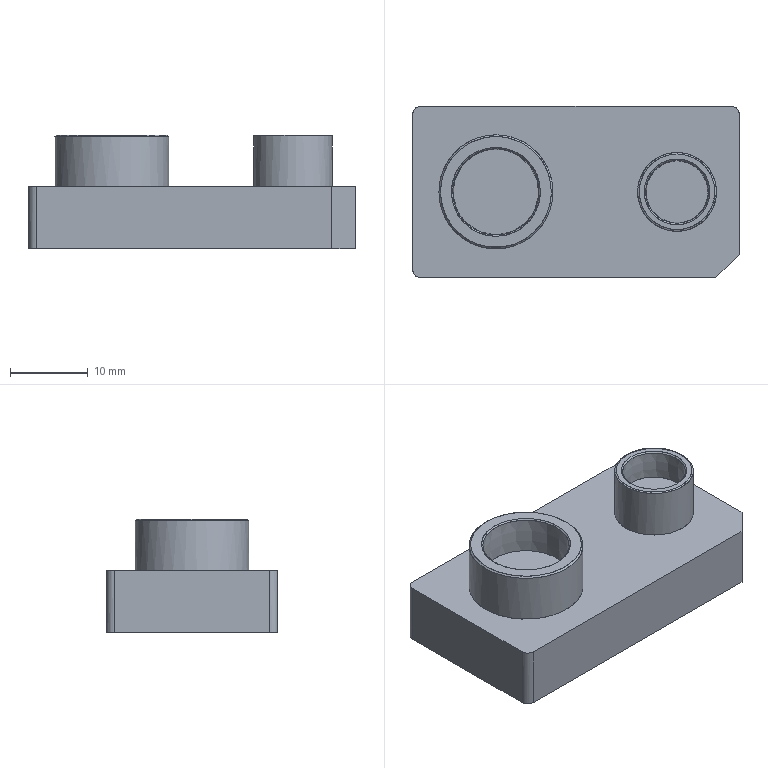NC program | PowerMill | posted by the shop | part box 42 x 22 x 14.621 mm
Lines 1 to 1559 of 126517:
%
G40 G49 G17 G80
( TOOL ID   D10C_1_1 )
( TOOL DIA. 10. TIP RAD 0 LENGTH 70.08 )
( Z = -.069 )
T1 M6
T2
G91 G28 Z0
G0 G90 G54
M08
S8000 M3
G0 X0 Y0 M8
G43 Z10.2 H1
X28.78 Y13.78
Z1.131
G1 Z-.069 F6000
X23.78 F10000
X-23.78
Y8.268
X23.78
Y2.756
X-23.78
Y-2.756
X23.78
Y-8.268
X-23.78
Y-13.78
X23.78
X28.78
G0 Z10.2
X.22 Y0
Z9.881
X31.126 Y5.112
Z.698
G1 Z-.502 F6000
X30.598 F10000
G3 X25.851 Y.364 I0 J-4.748
G1 Y-14.113
G2 X24.851 Y-15.113 I-1. J0
G1 X-24.411
G2 X-25.411 Y-14.113 I0 J1.
G1 Y14.113
G2 X-24.411 Y15.113 I1. J0
G1 X24.851
G2 X25.851 Y14.113 I0 J-1.
G1 Y.364
X23.346 Y.387
X23.339 Y-.387
X23.288 Y-1.16
X23.165 Y-1.934
X22.993 Y-2.707
X22.744 Y-3.48
X22.439 Y-4.254
X22.039 Y-5.027
X21.574 Y-5.801
X20.989 Y-6.574
X20.329 Y-7.311
X19.556 Y-8.014
X18.782 Y-8.573
X18.009 Y-9.061
X17.235 Y-9.439
X16.701 Y-9.668
X15.689 Y-9.993
X14.915 Y-10.175
X14.142 Y-10.285
X13.368 Y-10.347
X12.595 Y-10.339
X11.821 Y-10.286
X11.048 Y-10.16
X10.275 Y-9.988
X9.501 Y-9.737
X8.728 Y-9.431
X7.954 Y-9.037
X7.181 Y-8.561
X6.581 Y-8.121
X5.722 Y-7.348
X5.001 Y-6.574
X4.426 Y-5.801
X4.087 Y-5.268
X3.561 Y-4.254
X3.314 Y-3.65
X3.007 Y-2.707
X2.837 Y-1.934
X2.712 Y-1.16
X2.661 Y-.387
X2.654 Y.387
X2.295
Y-.387
X2.248 Y-1.16
X2.153 Y-1.934
X2.008 Y-2.707
X1.812 Y-3.48
X1.562 Y-4.254
X1.256 Y-5.027
X.993 Y-5.601
X.458 Y-6.574
X-.052 Y-7.348
X-.553 Y-8.001
X-1.327 Y-8.853
X-2.1 Y-9.578
X-2.874 Y-10.193
X-3.647 Y-10.713
X-4.421 Y-11.154
X-5.194 Y-11.527
X-6.381 Y-11.988
X-7.514 Y-12.294
X-8.288 Y-12.445
X-9.061 Y-12.546
X-9.835 Y-12.599
X-10.608 Y-12.605
X-11.381 Y-12.563
X-12.155 Y-12.473
X-12.928 Y-12.334
X-14.227 Y-11.988
X-15.249 Y-11.598
X-16.063 Y-11.215
X-16.795 Y-10.809
X-17.569 Y-10.31
X-18.342 Y-9.721
X-19.116 Y-9.021
X-19.889 Y-8.196
X-20.557 Y-7.348
X-21.066 Y-6.574
X-21.436 Y-5.929
X-21.865 Y-5.027
X-22.209 Y-4.156
X-22.421 Y-3.48
X-22.617 Y-2.707
X-22.762 Y-1.934
X-22.857 Y-1.16
X-22.904 Y-.387
Y.387
X-22.857 Y1.16
X-22.762 Y1.934
X-22.617 Y2.707
X-22.421 Y3.48
X-22.209 Y4.156
X-21.865 Y5.027
X-21.436 Y5.929
X-21.066 Y6.574
X-20.663 Y7.191
X-19.955 Y8.121
X-19.238 Y8.894
X-18.406 Y9.668
X-17.569 Y10.31
X-16.795 Y10.809
X-16.063 Y11.215
X-15.249 Y11.598
X-14.227 Y11.988
X-12.928 Y12.334
X-12.155 Y12.473
X-11.381 Y12.563
X-10.608 Y12.605
X-9.835 Y12.599
X-9.061 Y12.546
X-8.288 Y12.445
X-7.514 Y12.294
X-6.381 Y11.988
X-5.194 Y11.527
X-4.421 Y11.154
X-3.647 Y10.713
X-2.874 Y10.193
X-2.203 Y9.668
X-1.327 Y8.853
X-.653 Y8.121
X-.052 Y7.348
X.458 Y6.574
X.89 Y5.801
X1.256 Y5.027
X1.562 Y4.254
X1.767 Y3.646
X2.008 Y2.707
X2.153 Y1.934
X2.248 Y1.16
X2.295 Y.387
X2.654
X2.718 Y1.16
X2.829 Y1.934
X3.013 Y2.707
X3.249 Y3.48
X3.57 Y4.254
X4.087 Y5.268
X4.861 Y6.397
X5.634 Y7.271
X6.407 Y7.974
X7.181 Y8.562
X7.715 Y8.894
X8.728 Y9.431
X9.501 Y9.737
X10.275 Y9.988
X11.048 Y10.161
X11.821 Y10.286
X12.595 Y10.338
X13.368 Y10.347
X14.142 Y10.281
X14.915 Y10.175
X15.689 Y9.989
X16.462 Y9.758
X17.235 Y9.44
X18.009 Y9.061
X18.782 Y8.586
X19.42 Y8.121
X20.293 Y7.348
X20.99 Y6.574
X21.574 Y5.801
X22.051 Y5.027
X22.432 Y4.254
X22.751 Y3.48
X22.985 Y2.707
X23.171 Y1.934
X23.28 Y1.16
X23.346 Y.387
X25.851 Y.364
G0 Z3.315
G1 X31.126 Y5.112
G0 Z.315
G1 Z-.885 F6000
X30.598 F10000
G3 X25.851 Y.364 I0 J-4.748
G1 Y-14.113
G2 X24.851 Y-15.113 I-1. J0
G1 X-24.411
G2 X-25.411 Y-14.113 I0 J1.
G1 Y14.113
G2 X-24.411 Y15.113 I1. J0
G1 X24.851
G2 X25.851 Y14.113 I0 J-1.
G1 Y.364
X23.346 Y.387
X23.339 Y-.387
X23.288 Y-1.16
X23.165 Y-1.934
X22.993 Y-2.707
X22.744 Y-3.48
X22.439 Y-4.254
X22.039 Y-5.027
X21.574 Y-5.801
X20.989 Y-6.574
X20.329 Y-7.311
X19.556 Y-8.014
X18.782 Y-8.573
X18.009 Y-9.061
X17.235 Y-9.44
X16.701 Y-9.668
X15.689 Y-9.993
X14.915 Y-10.175
X14.142 Y-10.285
X13.368 Y-10.347
X12.595 Y-10.339
X11.821 Y-10.286
X11.048 Y-10.16
X10.275 Y-9.988
X9.501 Y-9.737
X8.728 Y-9.431
X7.954 Y-9.037
X7.181 Y-8.561
X6.581 Y-8.121
X5.722 Y-7.348
X5.001 Y-6.574
X4.426 Y-5.801
X4.087 Y-5.268
X3.561 Y-4.254
X3.314 Y-3.65
X3.007 Y-2.707
X2.837 Y-1.934
X2.712 Y-1.16
X2.661 Y-.387
X2.654 Y.387
X2.295
Y-.387
X2.248 Y-1.16
X2.153 Y-1.934
X2.008 Y-2.707
X1.812 Y-3.48
X1.562 Y-4.254
X1.256 Y-5.027
X.993 Y-5.601
X.458 Y-6.574
X-.052 Y-7.348
X-.553 Y-8.001
X-1.327 Y-8.853
X-2.1 Y-9.578
X-2.874 Y-10.193
X-3.647 Y-10.713
X-4.421 Y-11.154
X-5.194 Y-11.527
X-6.381 Y-11.988
X-7.514 Y-12.294
X-8.288 Y-12.445
X-9.061 Y-12.546
X-9.835 Y-12.599
X-10.608 Y-12.605
X-11.381 Y-12.563
X-12.155 Y-12.473
X-12.928 Y-12.334
X-14.227 Y-11.988
X-15.249 Y-11.598
X-16.063 Y-11.215
X-16.795 Y-10.809
X-17.569 Y-10.31
X-18.342 Y-9.721
X-19.116 Y-9.021
X-19.889 Y-8.196
X-20.557 Y-7.348
X-21.066 Y-6.574
X-21.436 Y-5.929
X-21.865 Y-5.027
X-22.209 Y-4.156
X-22.421 Y-3.48
X-22.617 Y-2.707
X-22.762 Y-1.934
X-22.857 Y-1.16
X-22.904 Y-.387
Y.387
X-22.857 Y1.16
X-22.762 Y1.934
X-22.617 Y2.707
X-22.421 Y3.48
X-22.209 Y4.156
X-21.865 Y5.027
X-21.436 Y5.929
X-21.066 Y6.574
X-20.663 Y7.191
X-19.955 Y8.121
X-19.238 Y8.894
X-18.406 Y9.668
X-17.569 Y10.31
X-16.795 Y10.809
X-16.063 Y11.215
X-15.249 Y11.598
X-14.227 Y11.988
X-12.928 Y12.334
X-12.155 Y12.473
X-11.381 Y12.563
X-10.608 Y12.605
X-9.835 Y12.599
X-9.061 Y12.546
X-8.288 Y12.445
X-7.514 Y12.294
X-6.381 Y11.988
X-5.194 Y11.527
X-4.421 Y11.154
X-3.647 Y10.713
X-2.874 Y10.193
X-2.203 Y9.668
X-1.327 Y8.853
X-.653 Y8.121
X-.052 Y7.348
X.458 Y6.574
X.89 Y5.801
X1.256 Y5.027
X1.562 Y4.254
X1.767 Y3.646
X2.008 Y2.707
X2.153 Y1.934
X2.248 Y1.16
X2.295 Y.387
X2.654
X2.718 Y1.16
X2.829 Y1.934
X3.013 Y2.707
X3.249 Y3.48
X3.57 Y4.254
X4.087 Y5.269
X4.861 Y6.397
X5.634 Y7.271
X6.407 Y7.974
X7.181 Y8.562
X7.715 Y8.894
X8.728 Y9.431
X9.501 Y9.737
X10.275 Y9.988
X11.048 Y10.161
X11.821 Y10.286
X12.595 Y10.338
X13.368 Y10.347
X14.142 Y10.281
X14.915 Y10.175
X15.689 Y9.989
X16.462 Y9.758
X17.235 Y9.44
X18.009 Y9.061
X18.782 Y8.586
X19.42 Y8.121
X20.293 Y7.348
X20.99 Y6.574
X21.574 Y5.801
X22.051 Y5.027
X22.432 Y4.254
X22.751 Y3.48
X22.985 Y2.707
X23.171 Y1.934
X23.28 Y1.16
X23.346 Y.387
X25.851 Y.364
G0 Z2.932
G1 X31.126 Y5.112
G0 Z-.068
G1 Z-1.268 F6000
X30.598 F10000
G3 X25.851 Y.364 I0 J-4.748
G1 Y-14.113
G2 X24.851 Y-15.113 I-1. J0
G1 X-24.411
G2 X-25.411 Y-14.113 I0 J1.
G1 Y14.113
G2 X-24.411 Y15.113 I1. J0
G1 X24.851
G2 X25.851 Y14.113 I0 J-1.
G1 Y.364
X23.346 Y.387
X23.339 Y-.387
X23.288 Y-1.16
X23.165 Y-1.934
X22.993 Y-2.707
X22.744 Y-3.48
X22.439 Y-4.254
X22.039 Y-5.027
X21.574 Y-5.801
X20.989 Y-6.574
X20.329 Y-7.311
X19.556 Y-8.014
X18.782 Y-8.573
X18.009 Y-9.061
X17.235 Y-9.44
X16.701 Y-9.668
X15.689 Y-9.993
X14.915 Y-10.175
X14.142 Y-10.285
X13.368 Y-10.347
X12.595 Y-10.339
X11.821 Y-10.286
X11.048 Y-10.16
X10.275 Y-9.988
X9.501 Y-9.737
X8.728 Y-9.431
X7.954 Y-9.037
X7.181 Y-8.561
X6.581 Y-8.121
X5.722 Y-7.348
X5.001 Y-6.574
X4.426 Y-5.801
X4.087 Y-5.268
X3.561 Y-4.254
X3.314 Y-3.65
X3.007 Y-2.707
X2.837 Y-1.934
X2.712 Y-1.16
X2.661 Y-.387
X2.654 Y.387
X2.295
Y-.387
X2.248 Y-1.16
X2.153 Y-1.934
X2.008 Y-2.707
X1.812 Y-3.48
X1.562 Y-4.254
X1.256 Y-5.027
X.993 Y-5.601
X.458 Y-6.574
X-.052 Y-7.348
X-.553 Y-8.001
X-1.327 Y-8.853
X-2.1 Y-9.578
X-2.874 Y-10.193
X-3.647 Y-10.713
X-4.421 Y-11.154
X-5.194 Y-11.527
X-6.381 Y-11.988
X-7.514 Y-12.294
X-8.288 Y-12.445
X-9.061 Y-12.546
X-9.835 Y-12.599
X-10.608 Y-12.605
X-11.381 Y-12.563
X-12.155 Y-12.473
X-12.928 Y-12.334
X-14.227 Y-11.988
X-15.249 Y-11.598
X-16.063 Y-11.215
X-16.795 Y-10.809
X-17.569 Y-10.31
X-18.342 Y-9.721
X-19.116 Y-9.021
X-19.889 Y-8.196
X-20.557 Y-7.348
X-21.066 Y-6.574
X-21.436 Y-5.929
X-21.865 Y-5.027
X-22.209 Y-4.156
X-22.421 Y-3.48
X-22.617 Y-2.707
X-22.762 Y-1.934
X-22.857 Y-1.16
X-22.904 Y-.387
Y.387
X-22.857 Y1.16
X-22.762 Y1.934
X-22.617 Y2.707
X-22.421 Y3.48
X-22.209 Y4.156
X-21.865 Y5.027
X-21.436 Y5.929
X-21.066 Y6.574
X-20.663 Y7.191
X-19.955 Y8.121
X-19.238 Y8.894
X-18.406 Y9.668
X-17.569 Y10.31
X-16.795 Y10.809
X-16.063 Y11.215
X-15.249 Y11.598
X-14.227 Y11.988
X-12.928 Y12.334
X-12.155 Y12.473
X-11.381 Y12.563
X-10.608 Y12.605
X-9.835 Y12.599
X-9.061 Y12.546
X-8.288 Y12.445
X-7.514 Y12.294
X-6.381 Y11.988
X-5.194 Y11.527
X-4.421 Y11.154
X-3.647 Y10.713
X-2.874 Y10.193
X-2.203 Y9.668
X-1.327 Y8.853
X-.653 Y8.121
X-.052 Y7.348
X.458 Y6.574
X.89 Y5.801
X1.256 Y5.027
X1.562 Y4.254
X1.767 Y3.646
X2.008 Y2.707
X2.153 Y1.934
X2.248 Y1.16
X2.295 Y.387
X2.654
X2.718 Y1.16
X2.829 Y1.934
X3.013 Y2.707
X3.249 Y3.48
X3.57 Y4.254
X4.087 Y5.269
X4.861 Y6.397
X5.634 Y7.271
X6.407 Y7.974
X7.181 Y8.562
X7.715 Y8.894
X8.728 Y9.431
X9.501 Y9.737
X10.275 Y9.988
X11.048 Y10.161
X11.821 Y10.286
X12.595 Y10.338
X13.368 Y10.347
X14.142 Y10.281
X14.915 Y10.175
X15.689 Y9.989
X16.462 Y9.758
X17.235 Y9.44
X18.009 Y9.061
X18.782 Y8.586
X19.42 Y8.121
X20.293 Y7.348
X20.99 Y6.574
X21.574 Y5.801
X22.051 Y5.027
X22.432 Y4.254
X22.751 Y3.48
X22.985 Y2.707
X23.171 Y1.934
X23.28 Y1.16
X23.346 Y.387
X25.851 Y.364
G0 Z2.549
G1 X31.126 Y5.112
G0 Z-.451
G1 Z-1.651 F6000
X30.598 F10000
G3 X25.851 Y.364 I0 J-4.748
G1 Y-14.113
G2 X24.851 Y-15.113 I-1. J0
G1 X-24.411
G2 X-25.411 Y-14.113 I0 J1.
G1 Y14.113
G2 X-24.411 Y15.113 I1. J0
G1 X24.851
G2 X25.851 Y14.113 I0 J-1.
G1 Y.364
X23.346 Y.387
X23.339 Y-.387
X23.288 Y-1.16
X23.165 Y-1.934
X22.993 Y-2.707
X22.744 Y-3.48
X22.439 Y-4.254
X22.039 Y-5.027
X21.574 Y-5.801
X20.989 Y-6.574
X20.329 Y-7.311
X19.556 Y-8.014
X18.782 Y-8.573
X18.009 Y-9.061
X17.235 Y-9.44
X16.701 Y-9.668
X15.689 Y-9.993
X14.915 Y-10.175
X14.142 Y-10.285
X13.368 Y-10.347
X12.595 Y-10.339
X11.821 Y-10.286
X11.048 Y-10.16
X10.275 Y-9.988
X9.501 Y-9.737
X8.728 Y-9.431
X7.954 Y-9.037
X7.181 Y-8.561
X6.581 Y-8.121
X5.722 Y-7.348
X5.001 Y-6.574
X4.426 Y-5.801
X4.087 Y-5.269
X3.561 Y-4.254
X3.314 Y-3.65
X3.007 Y-2.707
X2.837 Y-1.934
X2.712 Y-1.16
X2.661 Y-.387
X2.654 Y.387
X2.295
Y-.387
X2.248 Y-1.16
X2.153 Y-1.934
X2.008 Y-2.707
X1.812 Y-3.48
X1.562 Y-4.254
X1.256 Y-5.027
X.993 Y-5.601
X.458 Y-6.574
X-.052 Y-7.348
X-.553 Y-8.001
X-1.327 Y-8.853
X-2.1 Y-9.578
X-2.874 Y-10.193
X-3.647 Y-10.713
X-4.421 Y-11.154
X-5.194 Y-11.527
X-6.381 Y-11.988
X-7.514 Y-12.294
X-8.288 Y-12.445
X-9.061 Y-12.546
X-9.835 Y-12.599
X-10.608 Y-12.605
X-11.381 Y-12.563
X-12.155 Y-12.473
X-12.928 Y-12.334
X-14.227 Y-11.988
X-15.249 Y-11.598
X-16.063 Y-11.215
X-16.795 Y-10.809
X-17.569 Y-10.31
X-18.342 Y-9.721
X-19.116 Y-9.021
X-19.889 Y-8.196
X-20.557 Y-7.348
X-21.066 Y-6.574
X-21.436 Y-5.929
X-21.865 Y-5.027
X-22.209 Y-4.156
X-22.421 Y-3.48
X-22.617 Y-2.707
X-22.762 Y-1.934
X-22.857 Y-1.16
X-22.904 Y-.387
Y.387
X-22.857 Y1.16
X-22.762 Y1.934
X-22.617 Y2.707
X-22.421 Y3.48
X-22.209 Y4.156
X-21.865 Y5.027
X-21.436 Y5.929
X-21.066 Y6.574
X-20.663 Y7.191
X-19.955 Y8.121
X-19.238 Y8.894
X-18.406 Y9.668
X-17.569 Y10.31
X-16.795 Y10.809
X-16.063 Y11.215
X-15.249 Y11.598
X-14.227 Y11.988
X-12.928 Y12.334
X-12.155 Y12.473
X-11.381 Y12.563
X-10.608 Y12.605
X-9.835 Y12.599
X-9.061 Y12.546
X-8.288 Y12.445
X-7.514 Y12.294
X-6.381 Y11.988
X-5.194 Y11.527
X-4.421 Y11.154
X-3.647 Y10.713
X-2.874 Y10.193
X-2.203 Y9.668
X-1.327 Y8.853
X-.653 Y8.121
X-.052 Y7.348
X.458 Y6.574
X.89 Y5.801
X1.256 Y5.027
X1.562 Y4.254
X1.767 Y3.646
X2.008 Y2.707
X2.153 Y1.934
X2.248 Y1.16
X2.295 Y.387
X2.654
X2.718 Y1.16
X2.829 Y1.934
X3.013 Y2.707
X3.249 Y3.48
X3.57 Y4.254
X4.087 Y5.269
X4.861 Y6.397
X5.634 Y7.271
X6.407 Y7.974
X7.181 Y8.562
X7.715 Y8.894
X8.728 Y9.431
X9.501 Y9.737
X10.275 Y9.988
X11.048 Y10.161
X11.821 Y10.286
X12.595 Y10.338
X13.368 Y10.347
X14.142 Y10.281
X14.915 Y10.175
X15.689 Y9.989
X16.462 Y9.758
X17.235 Y9.44
X18.009 Y9.061
X18.782 Y8.586
X19.42 Y8.121
X20.293 Y7.348
X20.99 Y6.574
X21.574 Y5.801
X22.051 Y5.027
X22.432 Y4.254
X22.751 Y3.48
X22.985 Y2.707
X23.171 Y1.934
X23.28 Y1.16
X23.346 Y.387
X25.851 Y.364
G0 Z2.166
G1 X31.126 Y5.112
G0 Z-.834
G1 Z-2.034 F6000
X30.598 F10000
G3 X25.851 Y.364 I0 J-4.748
G1 Y-14.113
G2 X24.851 Y-15.113 I-1. J0
G1 X-24.411
G2 X-25.411 Y-14.113 I0 J1.
G1 Y14.113
G2 X-24.411 Y15.113 I1. J0
G1 X24.851
G2 X25.851 Y14.113 I0 J-1.
G1 Y.364
X23.346 Y.387
X23.339 Y-.387
X23.288 Y-1.16
X23.165 Y-1.934
X22.993 Y-2.707
X22.744 Y-3.48
X22.439 Y-4.254
X22.039 Y-5.027
X21.574 Y-5.801
X20.989 Y-6.574
X20.329 Y-7.311
X19.556 Y-8.014
X18.782 Y-8.573
X18.009 Y-9.061
X17.235 Y-9.44
X16.701 Y-9.668
X15.689 Y-9.993
X14.915 Y-10.175
X14.142 Y-10.285
X13.368 Y-10.347
X12.595 Y-10.339
X11.821 Y-10.286
X11.048 Y-10.16
X10.275 Y-9.988
X9.501 Y-9.737
X8.728 Y-9.431
X7.954 Y-9.037
X7.181 Y-8.561
X6.581 Y-8.121
X5.722 Y-7.348
X5.001 Y-6.574
X4.426 Y-5.801
X4.087 Y-5.269
X3.561 Y-4.254
X3.314 Y-3.65
X3.007 Y-2.707
X2.837 Y-1.934
X2.712 Y-1.16
X2.661 Y-.387
X2.654 Y.387
X2.295
Y-.387
X2.248 Y-1.16
X2.153 Y-1.934
X2.008 Y-2.707
X1.812 Y-3.48
X1.562 Y-4.254
X1.256 Y-5.027
X.993 Y-5.601
X.458 Y-6.574
X-.052 Y-7.348
X-.553 Y-8.001
X-1.327 Y-8.853
X-2.1 Y-9.578
X-2.874 Y-10.193
X-3.647 Y-10.713
X-4.421 Y-11.154
X-5.194 Y-11.527
X-6.381 Y-11.988
X-7.514 Y-12.294
X-8.288 Y-12.445
X-9.061 Y-12.546
X-9.835 Y-12.599
X-10.608 Y-12.605
X-11.381 Y-12.563
X-12.155 Y-12.473
X-12.928 Y-12.334
X-14.227 Y-11.988
X-15.249 Y-11.598
X-16.063 Y-11.215
X-16.795 Y-10.809
X-17.569 Y-10.31
X-18.342 Y-9.721
X-19.116 Y-9.021
X-19.889 Y-8.196
X-20.557 Y-7.348
X-21.066 Y-6.574
X-21.436 Y-5.929
X-21.865 Y-5.027
X-22.209 Y-4.156
X-22.421 Y-3.48
X-22.617 Y-2.707
X-22.762 Y-1.934
X-22.857 Y-1.16
X-22.904 Y-.387
Y.387
X-22.857 Y1.16
X-22.762 Y1.934
X-22.617 Y2.707
X-22.421 Y3.48
X-22.209 Y4.156
X-21.865 Y5.027
X-21.436 Y5.929
X-21.066 Y6.574
X-20.663 Y7.191
X-19.955 Y8.121
X-19.238 Y8.894
X-18.406 Y9.668
X-17.569 Y10.31
X-16.795 Y10.809
X-16.063 Y11.215
X-15.249 Y11.598
X-14.227 Y11.988
X-12.928 Y12.334
X-12.155 Y12.473
X-11.381 Y12.563
X-10.608 Y12.605
X-9.835 Y12.599
X-9.061 Y12.546
X-8.288 Y12.445
X-7.514 Y12.294
X-6.381 Y11.988
X-5.194 Y11.527
X-4.421 Y11.154
X-3.647 Y10.713
X-2.874 Y10.193
X-2.203 Y9.668
X-1.327 Y8.853
X-.653 Y8.121
X-.052 Y7.348
X.458 Y6.574
X.89 Y5.801
X1.256 Y5.027
X1.562 Y4.254
X1.767 Y3.646
X2.008 Y2.707
X2.153 Y1.934
X2.248 Y1.16
X2.295 Y.387
X2.654
X2.718 Y1.16
X2.829 Y1.934
X3.013 Y2.707
X3.249 Y3.48
X3.57 Y4.254
X4.087 Y5.269
X4.861 Y6.397
X5.634 Y7.271
X6.407 Y7.974
X7.181 Y8.562
X7.715 Y8.894
X8.728 Y9.431
X9.501 Y9.737
X10.275 Y9.988
X11.048 Y10.161
X11.821 Y10.286
X12.595 Y10.338
X13.368 Y10.347
X14.142 Y10.281
X14.915 Y10.175
X15.689 Y9.989
X16.462 Y9.758
X17.235 Y9.44
X18.009 Y9.061
X18.782 Y8.586
X19.42 Y8.121
X20.293 Y7.348
X20.99 Y6.574
X21.574 Y5.801
X22.051 Y5.027
X22.432 Y4.254
X22.751 Y3.48
X22.985 Y2.707
X23.171 Y1.934
X23.28 Y1.16
X23.346 Y.387
X25.851 Y.364
G0 Z1.783
G1 X31.126 Y5.112
G0 Z-1.217
G1 Z-2.417 F6000
X30.598 F10000
G3 X25.851 Y.364 I0 J-4.748
G1 Y-14.113
G2 X24.851 Y-15.113 I-1. J0
G1 X-24.411
G2 X-25.411 Y-14.113 I0 J1.
G1 Y14.113
G2 X-24.411 Y15.113 I1. J0
G1 X24.851
G2 X25.851 Y14.113 I0 J-1.
G1 Y.364
X23.346 Y.387
X23.339 Y-.387
X23.288 Y-1.16
X23.165 Y-1.934
X22.993 Y-2.707
X22.744 Y-3.48
X22.439 Y-4.254
X22.039 Y-5.027
X21.574 Y-5.801
X20.989 Y-6.574
X20.329 Y-7.311
X19.556 Y-8.014
X18.782 Y-8.573
X18.009 Y-9.061
X17.235 Y-9.44
X16.701 Y-9.668
X15.689 Y-9.993
X14.915 Y-10.175
X14.142 Y-10.285
X13.368 Y-10.347
X12.595 Y-10.339
X11.821 Y-10.286
X11.048 Y-10.16
X10.275 Y-9.988
X9.501 Y-9.737
X8.728 Y-9.431
X7.954 Y-9.037
X7.181 Y-8.561
X6.581 Y-8.121
X5.722 Y-7.348
X5.001 Y-6.574
X4.426 Y-5.801
X4.087 Y-5.269
X3.561 Y-4.254
X3.314 Y-3.65
X3.007 Y-2.707
X2.837 Y-1.934
X2.712 Y-1.16
X2.661 Y-.387
X2.654 Y.387
X2.295
Y-.387
X2.248 Y-1.16
X2.153 Y-1.934
X2.008 Y-2.707
X1.812 Y-3.48
X1.562 Y-4.254
X1.256 Y-5.027
X.993 Y-5.601
X.458 Y-6.574
X-.052 Y-7.348
X-.553 Y-8.001
X-1.327 Y-8.853
X-2.1 Y-9.578
X-2.874 Y-10.193
X-3.647 Y-10.713
X-4.421 Y-11.154
X-5.194 Y-11.527
X-6.381 Y-11.988
X-7.514 Y-12.294
X-8.288 Y-12.445
X-9.061 Y-12.546
X-9.835 Y-12.599
X-10.608 Y-12.605
X-11.381 Y-12.563
X-12.155 Y-12.473
X-12.928 Y-12.334
X-14.227 Y-11.988
X-15.249 Y-11.598
X-16.063 Y-11.215
X-16.795 Y-10.809
X-17.569 Y-10.31
X-18.342 Y-9.721
X-19.116 Y-9.021
X-19.889 Y-8.196
X-20.557 Y-7.348
X-21.066 Y-6.574
X-21.436 Y-5.929
X-21.865 Y-5.027
X-22.209 Y-4.156
X-22.421 Y-3.48
X-22.617 Y-2.707
X-22.762 Y-1.934
X-22.857 Y-1.16
X-22.904 Y-.387
Y.387
X-22.857 Y1.16
X-22.762 Y1.934
X-22.617 Y2.707
X-22.421 Y3.48
X-22.209 Y4.156
X-21.865 Y5.027
X-21.436 Y5.929
X-21.066 Y6.574
X-20.663 Y7.191
X-19.955 Y8.121
X-19.238 Y8.894
X-18.406 Y9.668
X-17.569 Y10.31
X-16.795 Y10.809
X-16.063 Y11.215
X-15.249 Y11.598
X-14.227 Y11.988
X-12.928 Y12.334
X-12.155 Y12.473
X-11.381 Y12.563
X-10.608 Y12.605
X-9.835 Y12.599
X-9.061 Y12.546
X-8.288 Y12.445
X-7.514 Y12.294
X-6.381 Y11.988
X-5.194 Y11.527
X-4.421 Y11.154
X-3.647 Y10.713
X-2.874 Y10.193
X-2.203 Y9.668
X-1.327 Y8.853
X-.653 Y8.121
X-.052 Y7.348
X.458 Y6.574
X.89 Y5.801
X1.256 Y5.027
X1.562 Y4.254
X1.767 Y3.646
X2.008 Y2.707
X2.153 Y1.934
X2.248 Y1.16
X2.295 Y.387
X2.654
X2.718 Y1.16
X2.829 Y1.934
X3.013 Y2.707
X3.249 Y3.48
X3.57 Y4.254
X4.087 Y5.269
X4.861 Y6.397
X5.634 Y7.271
X6.407 Y7.974
X7.181 Y8.562
X7.715 Y8.894
X8.728 Y9.431
X9.501 Y9.737
X10.275 Y9.988
X11.048 Y10.161
X11.821 Y10.286
X12.595 Y10.338
X13.368 Y10.347
X14.142 Y10.281
X14.915 Y10.175
X15.689 Y9.989
X16.462 Y9.758
X17.235 Y9.44
X18.009 Y9.061
X18.782 Y8.586
X19.42 Y8.121
X20.293 Y7.348
X20.99 Y6.574
X21.574 Y5.801
X22.051 Y5.027
X22.432 Y4.254
X22.751 Y3.48
X22.985 Y2.707
X23.171 Y1.934
X23.28 Y1.16
X23.346 Y.387
X25.851 Y.364
G0 Z1.4
G1 X31.126 Y5.112
G0 Z-1.6
G1 Z-2.8 F6000
X30.598 F10000
G3 X25.851 Y.364 I0 J-4.748
G1 Y-14.113
G2 X24.851 Y-15.113 I-1. J0
G1 X-24.411
G2 X-25.411 Y-14.113 I0 J1.
G1 Y14.113
G2 X-24.411 Y15.113 I1. J0
G1 X24.851
G2 X25.851 Y14.113 I0 J-1.
G1 Y.364
X23.346 Y.387
X23.339 Y-.387
X23.288 Y-1.16
X23.165 Y-1.934
X22.993 Y-2.707
X22.744 Y-3.48
X22.439 Y-4.254
X22.039 Y-5.027
X21.574 Y-5.801
X20.989 Y-6.574
X20.329 Y-7.311
X19.556 Y-8.014
X18.782 Y-8.573
X18.009 Y-9.061
X17.235 Y-9.44
X16.701 Y-9.668
X15.689 Y-9.993
X14.915 Y-10.175
X14.142 Y-10.285
X13.368 Y-10.347
X12.595 Y-10.339
X11.821 Y-10.286
X11.048 Y-10.16
X10.275 Y-9.988
X9.501 Y-9.737
X8.728 Y-9.431
X7.954 Y-9.037
X7.181 Y-8.561
X6.581 Y-8.121
X5.722 Y-7.348
X5.001 Y-6.574
X4.426 Y-5.801
X4.087 Y-5.269
X3.561 Y-4.254
X3.314 Y-3.65
X3.007 Y-2.707
X2.837 Y-1.934
X2.712 Y-1.16
X2.661 Y-.387
X2.654 Y.387
X2.295
Y-.387
X2.248 Y-1.16
X2.153 Y-1.934
X2.008 Y-2.707
X1.812 Y-3.48
X1.562 Y-4.254
X1.256 Y-5.027
X.993 Y-5.601
X.458 Y-6.574
X-.052 Y-7.348
X-.553 Y-8.001
X-1.327 Y-8.853
X-2.1 Y-9.578
X-2.874 Y-10.193
X-3.647 Y-10.713
X-4.421 Y-11.154
X-5.194 Y-11.527
X-6.381 Y-11.988
X-7.514 Y-12.294
X-8.288 Y-12.445
X-9.061 Y-12.546
X-9.835 Y-12.599
X-10.608 Y-12.605
X-11.381 Y-12.563
X-12.155 Y-12.473
X-12.928 Y-12.334
X-14.228 Y-11.988
X-15.249 Y-11.598
X-16.063 Y-11.215
X-16.795 Y-10.809
X-17.569 Y-10.31
X-18.342 Y-9.721
X-19.116 Y-9.021
X-19.889 Y-8.196
X-20.557 Y-7.348
X-21.066 Y-6.574
X-21.436 Y-5.929
X-21.865 Y-5.027
X-22.209 Y-4.156
X-22.421 Y-3.48
X-22.617 Y-2.707
X-22.762 Y-1.934
X-22.857 Y-1.16
X-22.904 Y-.387
Y.387
X-22.857 Y1.16
X-22.762 Y1.934
X-22.617 Y2.707
X-22.421 Y3.48
X-22.209 Y4.156
X-21.865 Y5.027
X-21.436 Y5.929
X-21.066 Y6.574
X-20.663 Y7.191
X-19.955 Y8.121
X-19.238 Y8.894
X-18.406 Y9.668
X-17.569 Y10.31
X-16.795 Y10.809
X-16.063 Y11.215
X-15.249 Y11.598
X-14.228 Y11.988
X-12.928 Y12.334
X-12.155 Y12.473
X-11.381 Y12.563
X-10.608 Y12.605
X-9.835 Y12.599
X-9.061 Y12.546
X-8.288 Y12.445
X-7.514 Y12.294
X-6.381 Y11.988
X-5.194 Y11.527
X-4.421 Y11.154
X-3.647 Y10.713
X-2.874 Y10.193
X-2.203 Y9.668
X-1.327 Y8.853
X-.653 Y8.121
X-.052 Y7.348
X.458 Y6.574
X.89 Y5.801
X1.256 Y5.027
X1.562 Y4.254
X1.767 Y3.646
X2.008 Y2.707
X2.153 Y1.934
X2.248 Y1.16
X2.295 Y.387
X2.654
X2.718 Y1.16
X2.829 Y1.934
X3.013 Y2.707
X3.249 Y3.48
X3.57 Y4.254
X4.087 Y5.269
X4.861 Y6.397
X5.634 Y7.271
X6.407 Y7.975
X7.181 Y8.562
X7.715 Y8.894
X8.728 Y9.431
X9.501 Y9.737
X10.275 Y9.988
X11.048 Y10.161
X11.821 Y10.286
X12.595 Y10.338
X13.368 Y10.347
X14.142 Y10.281
X14.915 Y10.175
X15.689 Y9.989
X16.462 Y9.758
X17.235 Y9.44
X18.009 Y9.061
X18.782 Y8.586
X19.42 Y8.121
X20.293 Y7.348
X20.99 Y6.574
X21.574 Y5.801
X22.051 Y5.027
X22.432 Y4.254
X22.751 Y3.48
X22.985 Y2.707
X23.171 Y1.934
X23.28 Y1.16
X23.346 Y.387
X25.851 Y.364
G0 Z1.017
G1 X31.126 Y5.112
G0 Z-1.983
G1 Z-3.183 F6000
X30.598 F10000
G3 X25.851 Y.364 I0 J-4.748
G1 Y-14.113
G2 X24.851 Y-15.113 I-1. J0
G1 X-24.411
G2 X-25.411 Y-14.113 I0 J1.
G1 Y14.113
G2 X-24.411 Y15.113 I1. J0
G1 X24.851
G2 X25.851 Y14.113 I0 J-1.
G1 Y.364
X23.346 Y.387
X23.339 Y-.387
X23.288 Y-1.16
X23.165 Y-1.934
X22.993 Y-2.707
X22.744 Y-3.48
X22.439 Y-4.254
X22.039 Y-5.027
X21.574 Y-5.801
X20.989 Y-6.574
X20.329 Y-7.311
X19.556 Y-8.014
X18.782 Y-8.573
X18.009 Y-9.061
X17.235 Y-9.44
X16.701 Y-9.668
X15.689 Y-9.993
X14.915 Y-10.175
X14.142 Y-10.285
X13.368 Y-10.347
X12.595 Y-10.339
X11.821 Y-10.286
X11.048 Y-10.16
X10.275 Y-9.988
X9.501 Y-9.737
X8.728 Y-9.431
X7.954 Y-9.037
X7.181 Y-8.561
X6.581 Y-8.121
X5.722 Y-7.348
X5.001 Y-6.574
X4.426 Y-5.801
X4.087 Y-5.269
X3.561 Y-4.254
X3.314 Y-3.65
X3.007 Y-2.707
X2.837 Y-1.934
X2.712 Y-1.16
X2.661 Y-.387
X2.654 Y.387
X2.295
Y-.387
X2.248 Y-1.16
X2.153 Y-1.934
X2.008 Y-2.707
X1.812 Y-3.48
X1.562 Y-4.254
X1.256 Y-5.027
X.993 Y-5.601
X.458 Y-6.574
X-.052 Y-7.348
X-.553 Y-8.001
X-1.327 Y-8.853
X-2.1 Y-9.578
X-2.874 Y-10.193
X-3.647 Y-10.713
X-4.421 Y-11.154
X-5.194 Y-11.527
X-6.381 Y-11.988
X-7.514 Y-12.294
X-8.288 Y-12.445
X-9.061 Y-12.546
X-9.835 Y-12.599
X-10.608 Y-12.605
X-11.381 Y-12.563
X-12.155 Y-12.473
X-12.928 Y-12.334
X-14.228 Y-11.988
X-15.249 Y-11.598
X-16.063 Y-11.215
X-16.795 Y-10.809
X-17.569 Y-10.31
X-18.342 Y-9.721
X-19.116 Y-9.021
X-19.889 Y-8.196
X-20.557 Y-7.348
X-21.066 Y-6.574
X-21.436 Y-5.929
X-21.865 Y-5.027
X-22.209 Y-4.156
X-22.421 Y-3.48
X-22.617 Y-2.707
X-22.762 Y-1.934
X-22.857 Y-1.16
X-22.904 Y-.387
Y.387
X-22.857 Y1.16
X-22.762 Y1.934
X-22.617 Y2.707
X-22.421 Y3.48
X-22.209 Y4.156
X-21.865 Y5.027
X-21.436 Y5.929
X-21.066 Y6.574
X-20.663 Y7.191
X-19.955 Y8.121
X-19.238 Y8.894
X-18.406 Y9.668
X-17.569 Y10.31
X-16.795 Y10.809
X-16.063 Y11.215
X-15.249 Y11.598
X-14.228 Y11.988
X-12.928 Y12.334
X-12.155 Y12.473
X-11.381 Y12.563
X-10.608 Y12.605
X-9.835 Y12.599
X-9.061 Y12.546
X-8.288 Y12.445
X-7.514 Y12.294
X-6.381 Y11.988
X-5.194 Y11.527
X-4.421 Y11.154
X-3.647 Y10.713
X-2.874 Y10.193
X-2.203 Y9.668
X-1.327 Y8.853
X-.653 Y8.121
X-.052 Y7.348
X.458 Y6.574
X.89 Y5.801
X1.256 Y5.027
X1.562 Y4.254
X1.767 Y3.646
X2.008 Y2.707
X2.153 Y1.934
X2.248 Y1.16
X2.295 Y.387
X2.654
X2.718 Y1.16
X2.829 Y1.934
X3.013 Y2.707
X3.249 Y3.48
X3.57 Y4.254
X4.087 Y5.269
X4.861 Y6.397
X5.634 Y7.271
X6.407 Y7.975
X7.181 Y8.562
X7.715 Y8.894
X8.728 Y9.431
X9.501 Y9.737
X10.275 Y9.988
X11.048 Y10.161
X11.821 Y10.286
X12.595 Y10.338
X13.368 Y10.347
X14.142 Y10.281
X14.915 Y10.175
X15.689 Y9.989
X16.462 Y9.758
X17.235 Y9.44
X18.009 Y9.061
X18.782 Y8.586
X19.42 Y8.121
X20.293 Y7.348
X20.99 Y6.574
X21.574 Y5.801
X22.051 Y5.027
X22.432 Y4.254
X22.751 Y3.48
X22.985 Y2.707
X23.171 Y1.934
X23.28 Y1.16
X23.346 Y.387
X25.851 Y.364
G0 Z.634
G1 X31.126 Y5.112
G0 Z-2.366
G1 Z-3.566 F6000
X30.598 F10000
G3 X25.851 Y.364 I0 J-4.748
G1 Y-14.113
G2 X24.851 Y-15.113 I-1. J0
G1 X-24.411
G2 X-25.411 Y-14.113 I0 J1.
G1 Y14.113
G2 X-24.411 Y15.113 I1. J0
G1 X24.851
G2 X25.851 Y14.113 I0 J-1.
G1 Y.364
X23.346 Y.387
X23.339 Y-.387
X23.288 Y-1.16
X23.165 Y-1.934
X22.993 Y-2.707
X22.744 Y-3.48
X22.439 Y-4.254
X22.039 Y-5.027
X21.574 Y-5.801
X20.989 Y-6.574
X20.329 Y-7.311
X19.556 Y-8.014
X18.782 Y-8.573
X18.009 Y-9.061
X17.235 Y-9.44
X16.701 Y-9.668
X15.689 Y-9.993
X14.915 Y-10.175
X14.142 Y-10.285
X13.368 Y-10.347
X12.595 Y-10.339
X11.821 Y-10.286
X11.048 Y-10.16
X10.275 Y-9.988
X9.501 Y-9.737
X8.728 Y-9.431
X7.954 Y-9.037
X7.181 Y-8.561
X6.581 Y-8.121
X5.722 Y-7.348
X5.001 Y-6.574
X4.426 Y-5.801
X4.087 Y-5.269
X3.561 Y-4.254
X3.314 Y-3.65
X3.007 Y-2.707
X2.837 Y-1.934
X2.712 Y-1.16
X2.661 Y-.387
X2.654 Y.387
X2.295
Y-.387
X2.248 Y-1.16
X2.153 Y-1.934
X2.008 Y-2.707
X1.812 Y-3.48
X1.562 Y-4.254
X1.256 Y-5.027
X.993 Y-5.601
X.458 Y-6.574
X-.052 Y-7.348
X-.553 Y-8.001
X-1.327 Y-8.853
X-2.1 Y-9.578
X-2.874 Y-10.193
X-3.647 Y-10.713